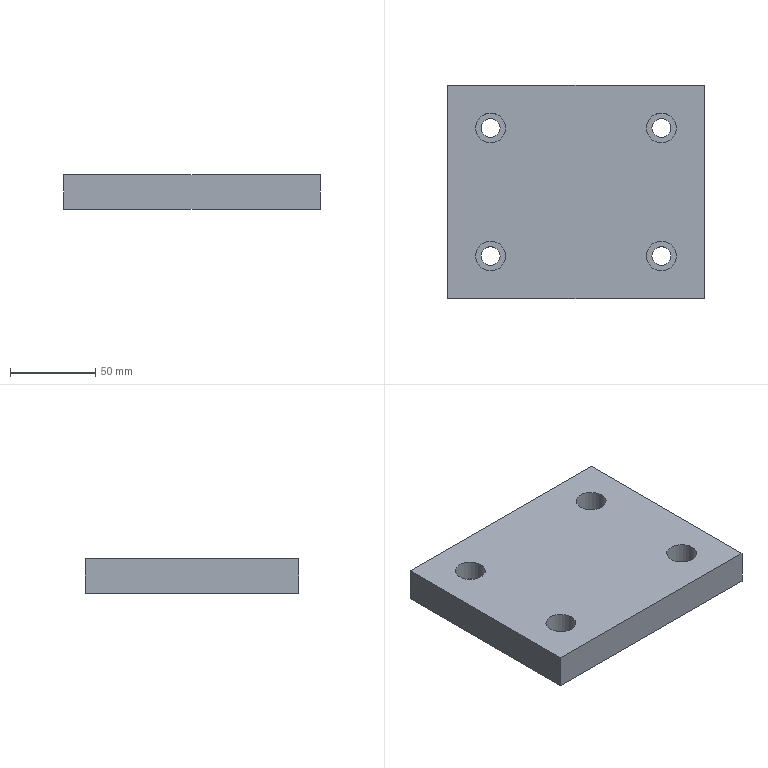Part | NX | features solid 2 | 1 solid | 18 faces | box 150 x 125 x 20 mm | volume 360414 mm3 | plane 10 | cylinder 8 | commonest cylinder face diameters 11 x4 17.5 x4
STEP:
#1=CARTESIAN_POINT('',(504.6,-600.,-350.));
#2=VERTEX_POINT('',#1);
#3=CARTESIAN_POINT('',(504.6,-600.,-370.));
#4=VERTEX_POINT('',#3);
#5=CARTESIAN_POINT('',(504.6,-600.,-350.));
#6=DIRECTION('',(0.,0.,1.));
#7=VECTOR('',#6,1000.);
#8=LINE('',#5,#7);
#9=EDGE_CURVE('',#2,#4,#8,.F.);
#10=ORIENTED_EDGE('',*,*,#9,.T.);
#11=CARTESIAN_POINT('',(354.6,-600.,-370.));
#12=VERTEX_POINT('',#11);
#13=CARTESIAN_POINT('',(504.6,-600.,-370.));
#14=DIRECTION('',(-1.,0.,0.));
#15=VECTOR('',#14,1000.);
#16=LINE('',#13,#15);
#17=EDGE_CURVE('',#4,#12,#16,.T.);
#18=ORIENTED_EDGE('',*,*,#17,.T.);
#19=CARTESIAN_POINT('',(354.6,-600.,-350.));
#20=VERTEX_POINT('',#19);
#21=CARTESIAN_POINT('',(354.6,-600.,-350.));
#22=DIRECTION('',(0.,0.,-1.));
#23=VECTOR('',#22,1000.);
#24=LINE('',#21,#23);
#25=EDGE_CURVE('',#20,#12,#24,.T.);
#26=ORIENTED_EDGE('',*,*,#25,.F.);
#27=CARTESIAN_POINT('',(504.6,-600.,-350.));
#28=DIRECTION('',(-1.,0.,0.));
#29=VECTOR('',#28,1000.);
#30=LINE('',#27,#29);
#31=EDGE_CURVE('',#2,#20,#30,.T.);
#32=ORIENTED_EDGE('',*,*,#31,.F.);
#33=EDGE_LOOP('',(#10,#18,#26,#32));
#34=FACE_BOUND('',#33,.T.);
#35=CARTESIAN_POINT('',(504.6,-600.,-350.));
#36=DIRECTION('',(0.,1.,0.));
#37=DIRECTION('',(-1.,0.,0.));
#38=AXIS2_PLACEMENT_3D('',#35,#36,#37);
#39=PLANE('',#38);
#40=ADVANCED_FACE('',(#34),#39,.T.);
#41=ORIENTED_EDGE('',*,*,#25,.T.);
#42=CARTESIAN_POINT('',(354.6,-725.,-370.));
#43=VERTEX_POINT('',#42);
#44=CARTESIAN_POINT('',(354.6,-600.,-370.));
#45=DIRECTION('',(0.,1.,0.));
#46=VECTOR('',#45,1000.);
#47=LINE('',#44,#46);
#48=EDGE_CURVE('',#12,#43,#47,.F.);
#49=ORIENTED_EDGE('',*,*,#48,.T.);
#50=CARTESIAN_POINT('',(354.6,-725.,-350.));
#51=VERTEX_POINT('',#50);
#52=CARTESIAN_POINT('',(354.6,-725.,-350.));
#53=DIRECTION('',(0.,0.,1.));
#54=VECTOR('',#53,1000.);
#55=LINE('',#52,#54);
#56=EDGE_CURVE('',#51,#43,#55,.F.);
#57=ORIENTED_EDGE('',*,*,#56,.F.);
#58=CARTESIAN_POINT('',(354.6,-600.,-350.));
#59=DIRECTION('',(0.,1.,0.));
#60=VECTOR('',#59,1000.);
#61=LINE('',#58,#60);
#62=EDGE_CURVE('',#20,#51,#61,.F.);
#63=ORIENTED_EDGE('',*,*,#62,.F.);
#64=EDGE_LOOP('',(#41,#49,#57,#63));
#65=FACE_BOUND('',#64,.T.);
#66=CARTESIAN_POINT('',(354.6,-600.,-350.));
#67=DIRECTION('',(-1.,0.,0.));
#68=DIRECTION('',(0.,-1.,0.));
#69=AXIS2_PLACEMENT_3D('',#66,#67,#68);
#70=PLANE('',#69);
#71=ADVANCED_FACE('',(#65),#70,.T.);
#72=ORIENTED_EDGE('',*,*,#56,.T.);
#73=CARTESIAN_POINT('',(504.6,-725.,-370.));
#74=VERTEX_POINT('',#73);
#75=CARTESIAN_POINT('',(504.6,-725.,-370.));
#76=DIRECTION('',(-1.,0.,0.));
#77=VECTOR('',#76,1000.);
#78=LINE('',#75,#77);
#79=EDGE_CURVE('',#74,#43,#78,.T.);
#80=ORIENTED_EDGE('',*,*,#79,.F.);
#81=CARTESIAN_POINT('',(504.6,-725.,-350.));
#82=VERTEX_POINT('',#81);
#83=CARTESIAN_POINT('',(504.6,-725.,-350.));
#84=DIRECTION('',(0.,0.,-1.));
#85=VECTOR('',#84,1000.);
#86=LINE('',#83,#85);
#87=EDGE_CURVE('',#82,#74,#86,.T.);
#88=ORIENTED_EDGE('',*,*,#87,.F.);
#89=CARTESIAN_POINT('',(504.6,-725.,-350.));
#90=DIRECTION('',(-1.,0.,0.));
#91=VECTOR('',#90,1000.);
#92=LINE('',#89,#91);
#93=EDGE_CURVE('',#82,#51,#92,.T.);
#94=ORIENTED_EDGE('',*,*,#93,.T.);
#95=EDGE_LOOP('',(#72,#80,#88,#94));
#96=FACE_BOUND('',#95,.T.);
#97=CARTESIAN_POINT('',(504.6,-725.,-350.));
#98=DIRECTION('',(0.,1.,0.));
#99=DIRECTION('',(-1.,0.,0.));
#100=AXIS2_PLACEMENT_3D('',#97,#98,#99);
#101=PLANE('',#100);
#102=ADVANCED_FACE('',(#96),#101,.F.);
#103=CARTESIAN_POINT('',(504.6,-600.,-350.));
#104=DIRECTION('',(0.,-1.,0.));
#105=VECTOR('',#104,1000.);
#106=LINE('',#103,#105);
#107=EDGE_CURVE('',#2,#82,#106,.T.);
#108=ORIENTED_EDGE('',*,*,#107,.T.);
#109=ORIENTED_EDGE('',*,*,#87,.T.);
#110=CARTESIAN_POINT('',(504.6,-600.,-370.));
#111=DIRECTION('',(0.,-1.,0.));
#112=VECTOR('',#111,1000.);
#113=LINE('',#110,#112);
#114=EDGE_CURVE('',#4,#74,#113,.T.);
#115=ORIENTED_EDGE('',*,*,#114,.F.);
#116=ORIENTED_EDGE('',*,*,#9,.F.);
#117=EDGE_LOOP('',(#108,#109,#115,#116));
#118=FACE_BOUND('',#117,.T.);
#119=CARTESIAN_POINT('',(504.6,-600.,-350.));
#120=DIRECTION('',(-1.,0.,0.));
#121=DIRECTION('',(0.,-1.,0.));
#122=AXIS2_PLACEMENT_3D('',#119,#120,#121);
#123=PLANE('',#122);
#124=ADVANCED_FACE('',(#118),#123,.F.);
#125=CARTESIAN_POINT('',(474.1,-625.,-370.));
#126=VERTEX_POINT('',#125);
#127=CARTESIAN_POINT('',(479.6,-625.,-370.));
#128=DIRECTION('',(0.,0.,1.));
#129=DIRECTION('',(-1.,0.,0.));
#130=AXIS2_PLACEMENT_3D('',#127,#128,#129);
#131=CIRCLE('',#130,5.5);
#132=EDGE_CURVE('',#126,#126,#131,.T.);
#133=ORIENTED_EDGE('',*,*,#132,.T.);
#134=EDGE_LOOP('',(#133));
#135=FACE_BOUND('',#134,.T.);
#136=CARTESIAN_POINT('',(374.1,-625.,-370.));
#137=VERTEX_POINT('',#136);
#138=CARTESIAN_POINT('',(379.6,-625.,-370.));
#139=DIRECTION('',(0.,0.,1.));
#140=DIRECTION('',(-1.,0.,0.));
#141=AXIS2_PLACEMENT_3D('',#138,#139,#140);
#142=CIRCLE('',#141,5.5);
#143=EDGE_CURVE('',#137,#137,#142,.T.);
#144=ORIENTED_EDGE('',*,*,#143,.T.);
#145=EDGE_LOOP('',(#144));
#146=FACE_BOUND('',#145,.T.);
#147=CARTESIAN_POINT('',(474.1,-700.,-370.));
#148=VERTEX_POINT('',#147);
#149=CARTESIAN_POINT('',(479.6,-700.,-370.));
#150=DIRECTION('',(0.,0.,-1.));
#151=DIRECTION('',(-1.,0.,0.));
#152=AXIS2_PLACEMENT_3D('',#149,#150,#151);
#153=CIRCLE('',#152,5.5);
#154=EDGE_CURVE('',#148,#148,#153,.F.);
#155=ORIENTED_EDGE('',*,*,#154,.T.);
#156=EDGE_LOOP('',(#155));
#157=FACE_BOUND('',#156,.T.);
#158=CARTESIAN_POINT('',(374.1,-700.,-370.));
#159=VERTEX_POINT('',#158);
#160=CARTESIAN_POINT('',(379.6,-700.,-370.));
#161=DIRECTION('',(0.,0.,-1.));
#162=DIRECTION('',(-1.,0.,0.));
#163=AXIS2_PLACEMENT_3D('',#160,#161,#162);
#164=CIRCLE('',#163,5.5);
#165=EDGE_CURVE('',#159,#159,#164,.F.);
#166=ORIENTED_EDGE('',*,*,#165,.T.);
#167=EDGE_LOOP('',(#166));
#168=FACE_BOUND('',#167,.T.);
#169=ORIENTED_EDGE('',*,*,#79,.T.);
#170=ORIENTED_EDGE('',*,*,#48,.F.);
#171=ORIENTED_EDGE('',*,*,#17,.F.);
#172=ORIENTED_EDGE('',*,*,#114,.T.);
#173=EDGE_LOOP('',(#169,#170,#171,#172));
#174=FACE_BOUND('',#173,.T.);
#175=CARTESIAN_POINT('',(504.6,-600.,-370.));
#176=DIRECTION('',(0.,0.,1.));
#177=DIRECTION('',(-1.,0.,0.));
#178=AXIS2_PLACEMENT_3D('',#175,#176,#177);
#179=PLANE('',#178);
#180=ADVANCED_FACE('',(#135,#146,#157,#168,#174),#179,.F.);
#181=CARTESIAN_POINT('',(488.35,-625.,-350.));
#182=VERTEX_POINT('',#181);
#183=CARTESIAN_POINT('',(479.6,-625.,-350.));
#184=DIRECTION('',(0.,0.,-1.));
#185=DIRECTION('',(1.,0.,0.));
#186=AXIS2_PLACEMENT_3D('',#183,#184,#185);
#187=CIRCLE('',#186,8.75);
#188=EDGE_CURVE('',#182,#182,#187,.T.);
#189=ORIENTED_EDGE('',*,*,#188,.T.);
#190=EDGE_LOOP('',(#189));
#191=FACE_BOUND('',#190,.T.);
#192=CARTESIAN_POINT('',(388.35,-625.,-350.));
#193=VERTEX_POINT('',#192);
#194=CARTESIAN_POINT('',(379.6,-625.,-350.));
#195=DIRECTION('',(0.,0.,-1.));
#196=DIRECTION('',(1.,0.,0.));
#197=AXIS2_PLACEMENT_3D('',#194,#195,#196);
#198=CIRCLE('',#197,8.75);
#199=EDGE_CURVE('',#193,#193,#198,.T.);
#200=ORIENTED_EDGE('',*,*,#199,.T.);
#201=EDGE_LOOP('',(#200));
#202=FACE_BOUND('',#201,.T.);
#203=CARTESIAN_POINT('',(470.85,-700.,-350.));
#204=VERTEX_POINT('',#203);
#205=CARTESIAN_POINT('',(479.6,-700.,-350.));
#206=DIRECTION('',(0.,0.,-1.));
#207=DIRECTION('',(-1.,0.,0.));
#208=AXIS2_PLACEMENT_3D('',#205,#206,#207);
#209=CIRCLE('',#208,8.75);
#210=EDGE_CURVE('',#204,#204,#209,.T.);
#211=ORIENTED_EDGE('',*,*,#210,.T.);
#212=EDGE_LOOP('',(#211));
#213=FACE_BOUND('',#212,.T.);
#214=CARTESIAN_POINT('',(370.85,-700.,-350.));
#215=VERTEX_POINT('',#214);
#216=CARTESIAN_POINT('',(379.6,-700.,-350.));
#217=DIRECTION('',(0.,0.,-1.));
#218=DIRECTION('',(-1.,0.,0.));
#219=AXIS2_PLACEMENT_3D('',#216,#217,#218);
#220=CIRCLE('',#219,8.75);
#221=EDGE_CURVE('',#215,#215,#220,.T.);
#222=ORIENTED_EDGE('',*,*,#221,.T.);
#223=EDGE_LOOP('',(#222));
#224=FACE_BOUND('',#223,.T.);
#225=ORIENTED_EDGE('',*,*,#93,.F.);
#226=ORIENTED_EDGE('',*,*,#107,.F.);
#227=ORIENTED_EDGE('',*,*,#31,.T.);
#228=ORIENTED_EDGE('',*,*,#62,.T.);
#229=EDGE_LOOP('',(#225,#226,#227,#228));
#230=FACE_BOUND('',#229,.T.);
#231=CARTESIAN_POINT('',(504.6,-600.,-350.));
#232=DIRECTION('',(0.,0.,1.));
#233=DIRECTION('',(-1.,0.,0.));
#234=AXIS2_PLACEMENT_3D('',#231,#232,#233);
#235=PLANE('',#234);
#236=ADVANCED_FACE('',(#191,#202,#213,#224,#230),#235,.T.);
#237=CARTESIAN_POINT('',(385.1,-700.,-362.));
#238=VERTEX_POINT('',#237);
#239=CARTESIAN_POINT('',(379.6,-700.,-362.));
#240=DIRECTION('',(0.,0.,-1.));
#241=DIRECTION('',(1.,0.,0.));
#242=AXIS2_PLACEMENT_3D('',#239,#240,#241);
#243=CIRCLE('',#242,5.5);
#244=EDGE_CURVE('',#238,#238,#243,.T.);
#245=ORIENTED_EDGE('',*,*,#244,.F.);
#246=EDGE_LOOP('',(#245));
#247=FACE_BOUND('',#246,.T.);
#248=ORIENTED_EDGE('',*,*,#165,.F.);
#249=EDGE_LOOP('',(#248));
#250=FACE_BOUND('',#249,.T.);
#251=CARTESIAN_POINT('',(379.6,-700.,-400.));
#252=DIRECTION('',(0.,0.,-1.));
#253=DIRECTION('',(1.,0.,0.));
#254=AXIS2_PLACEMENT_3D('',#251,#252,#253);
#255=CYLINDRICAL_SURFACE('',#254,5.5);
#256=ADVANCED_FACE('',(#247,#250),#255,.F.);
#257=ORIENTED_EDGE('',*,*,#244,.T.);
#258=EDGE_LOOP('',(#257));
#259=FACE_BOUND('',#258,.T.);
#260=CARTESIAN_POINT('',(388.35,-700.,-362.));
#261=VERTEX_POINT('',#260);
#262=CARTESIAN_POINT('',(379.6,-700.,-362.));
#263=DIRECTION('',(0.,0.,-1.));
#264=DIRECTION('',(1.,0.,0.));
#265=AXIS2_PLACEMENT_3D('',#262,#263,#264);
#266=CIRCLE('',#265,8.75);
#267=EDGE_CURVE('',#261,#261,#266,.T.);
#268=ORIENTED_EDGE('',*,*,#267,.F.);
#269=EDGE_LOOP('',(#268));
#270=FACE_BOUND('',#269,.T.);
#271=CARTESIAN_POINT('',(417.1,-700.,-362.));
#272=DIRECTION('',(0.,0.,-1.));
#273=DIRECTION('',(1.,0.,0.));
#274=AXIS2_PLACEMENT_3D('',#271,#272,#273);
#275=PLANE('',#274);
#276=ADVANCED_FACE('',(#259,#270),#275,.F.);
#277=ORIENTED_EDGE('',*,*,#267,.T.);
#278=EDGE_LOOP('',(#277));
#279=FACE_BOUND('',#278,.T.);
#280=ORIENTED_EDGE('',*,*,#221,.F.);
#281=EDGE_LOOP('',(#280));
#282=FACE_BOUND('',#281,.T.);
#283=CARTESIAN_POINT('',(379.6,-700.,-350.));
#284=DIRECTION('',(0.,0.,-1.));
#285=DIRECTION('',(1.,0.,0.));
#286=AXIS2_PLACEMENT_3D('',#283,#284,#285);
#287=CYLINDRICAL_SURFACE('',#286,8.75);
#288=ADVANCED_FACE('',(#279,#282),#287,.F.);
#289=CARTESIAN_POINT('',(485.1,-700.,-362.));
#290=VERTEX_POINT('',#289);
#291=CARTESIAN_POINT('',(479.6,-700.,-362.));
#292=DIRECTION('',(0.,0.,-1.));
#293=DIRECTION('',(1.,0.,0.));
#294=AXIS2_PLACEMENT_3D('',#291,#292,#293);
#295=CIRCLE('',#294,5.5);
#296=EDGE_CURVE('',#290,#290,#295,.T.);
#297=ORIENTED_EDGE('',*,*,#296,.F.);
#298=EDGE_LOOP('',(#297));
#299=FACE_BOUND('',#298,.T.);
#300=ORIENTED_EDGE('',*,*,#154,.F.);
#301=EDGE_LOOP('',(#300));
#302=FACE_BOUND('',#301,.T.);
#303=CARTESIAN_POINT('',(479.6,-700.,-400.));
#304=DIRECTION('',(0.,0.,-1.));
#305=DIRECTION('',(1.,0.,0.));
#306=AXIS2_PLACEMENT_3D('',#303,#304,#305);
#307=CYLINDRICAL_SURFACE('',#306,5.5);
#308=ADVANCED_FACE('',(#299,#302),#307,.F.);
#309=ORIENTED_EDGE('',*,*,#296,.T.);
#310=EDGE_LOOP('',(#309));
#311=FACE_BOUND('',#310,.T.);
#312=CARTESIAN_POINT('',(488.35,-700.,-362.));
#313=VERTEX_POINT('',#312);
#314=CARTESIAN_POINT('',(479.6,-700.,-362.));
#315=DIRECTION('',(0.,0.,-1.));
#316=DIRECTION('',(1.,0.,0.));
#317=AXIS2_PLACEMENT_3D('',#314,#315,#316);
#318=CIRCLE('',#317,8.75);
#319=EDGE_CURVE('',#313,#313,#318,.T.);
#320=ORIENTED_EDGE('',*,*,#319,.F.);
#321=EDGE_LOOP('',(#320));
#322=FACE_BOUND('',#321,.T.);
#323=CARTESIAN_POINT('',(467.1,-700.,-362.));
#324=DIRECTION('',(0.,0.,-1.));
#325=DIRECTION('',(1.,0.,0.));
#326=AXIS2_PLACEMENT_3D('',#323,#324,#325);
#327=PLANE('',#326);
#328=ADVANCED_FACE('',(#311,#322),#327,.F.);
#329=ORIENTED_EDGE('',*,*,#319,.T.);
#330=EDGE_LOOP('',(#329));
#331=FACE_BOUND('',#330,.T.);
#332=ORIENTED_EDGE('',*,*,#210,.F.);
#333=EDGE_LOOP('',(#332));
#334=FACE_BOUND('',#333,.T.);
#335=CARTESIAN_POINT('',(479.6,-700.,-350.));
#336=DIRECTION('',(0.,0.,-1.));
#337=DIRECTION('',(1.,0.,0.));
#338=AXIS2_PLACEMENT_3D('',#335,#336,#337);
#339=CYLINDRICAL_SURFACE('',#338,8.75);
#340=ADVANCED_FACE('',(#331,#334),#339,.F.);
#341=CARTESIAN_POINT('',(385.1,-625.,-362.));
#342=VERTEX_POINT('',#341);
#343=CARTESIAN_POINT('',(379.6,-625.,-362.));
#344=DIRECTION('',(0.,0.,-1.));
#345=DIRECTION('',(1.,0.,0.));
#346=AXIS2_PLACEMENT_3D('',#343,#344,#345);
#347=CIRCLE('',#346,5.5);
#348=EDGE_CURVE('',#342,#342,#347,.T.);
#349=ORIENTED_EDGE('',*,*,#348,.F.);
#350=EDGE_LOOP('',(#349));
#351=FACE_BOUND('',#350,.T.);
#352=ORIENTED_EDGE('',*,*,#143,.F.);
#353=EDGE_LOOP('',(#352));
#354=FACE_BOUND('',#353,.T.);
#355=CARTESIAN_POINT('',(379.6,-625.,-400.));
#356=DIRECTION('',(0.,0.,-1.));
#357=DIRECTION('',(1.,0.,0.));
#358=AXIS2_PLACEMENT_3D('',#355,#356,#357);
#359=CYLINDRICAL_SURFACE('',#358,5.5);
#360=ADVANCED_FACE('',(#351,#354),#359,.F.);
#361=ORIENTED_EDGE('',*,*,#348,.T.);
#362=EDGE_LOOP('',(#361));
#363=FACE_BOUND('',#362,.T.);
#364=CARTESIAN_POINT('',(388.35,-625.,-362.));
#365=VERTEX_POINT('',#364);
#366=CARTESIAN_POINT('',(379.6,-625.,-362.));
#367=DIRECTION('',(0.,0.,-1.));
#368=DIRECTION('',(1.,0.,0.));
#369=AXIS2_PLACEMENT_3D('',#366,#367,#368);
#370=CIRCLE('',#369,8.75);
#371=EDGE_CURVE('',#365,#365,#370,.T.);
#372=ORIENTED_EDGE('',*,*,#371,.F.);
#373=EDGE_LOOP('',(#372));
#374=FACE_BOUND('',#373,.T.);
#375=CARTESIAN_POINT('',(417.1,-625.,-362.));
#376=DIRECTION('',(0.,0.,-1.));
#377=DIRECTION('',(1.,0.,0.));
#378=AXIS2_PLACEMENT_3D('',#375,#376,#377);
#379=PLANE('',#378);
#380=ADVANCED_FACE('',(#363,#374),#379,.F.);
#381=ORIENTED_EDGE('',*,*,#371,.T.);
#382=EDGE_LOOP('',(#381));
#383=FACE_BOUND('',#382,.T.);
#384=ORIENTED_EDGE('',*,*,#199,.F.);
#385=EDGE_LOOP('',(#384));
#386=FACE_BOUND('',#385,.T.);
#387=CARTESIAN_POINT('',(379.6,-625.,-350.));
#388=DIRECTION('',(0.,0.,-1.));
#389=DIRECTION('',(1.,0.,0.));
#390=AXIS2_PLACEMENT_3D('',#387,#388,#389);
#391=CYLINDRICAL_SURFACE('',#390,8.75);
#392=ADVANCED_FACE('',(#383,#386),#391,.F.);
#393=CARTESIAN_POINT('',(485.1,-625.,-362.));
#394=VERTEX_POINT('',#393);
#395=CARTESIAN_POINT('',(479.6,-625.,-362.));
#396=DIRECTION('',(0.,0.,-1.));
#397=DIRECTION('',(1.,0.,0.));
#398=AXIS2_PLACEMENT_3D('',#395,#396,#397);
#399=CIRCLE('',#398,5.5);
#400=EDGE_CURVE('',#394,#394,#399,.T.);
#401=ORIENTED_EDGE('',*,*,#400,.F.);
#402=EDGE_LOOP('',(#401));
#403=FACE_BOUND('',#402,.T.);
#404=ORIENTED_EDGE('',*,*,#132,.F.);
#405=EDGE_LOOP('',(#404));
#406=FACE_BOUND('',#405,.T.);
#407=CARTESIAN_POINT('',(479.6,-625.,-400.));
#408=DIRECTION('',(0.,0.,-1.));
#409=DIRECTION('',(1.,0.,0.));
#410=AXIS2_PLACEMENT_3D('',#407,#408,#409);
#411=CYLINDRICAL_SURFACE('',#410,5.5);
#412=ADVANCED_FACE('',(#403,#406),#411,.F.);
#413=ORIENTED_EDGE('',*,*,#400,.T.);
#414=EDGE_LOOP('',(#413));
#415=FACE_BOUND('',#414,.T.);
#416=CARTESIAN_POINT('',(488.35,-625.,-362.));
#417=VERTEX_POINT('',#416);
#418=CARTESIAN_POINT('',(479.6,-625.,-362.));
#419=DIRECTION('',(0.,0.,-1.));
#420=DIRECTION('',(1.,0.,0.));
#421=AXIS2_PLACEMENT_3D('',#418,#419,#420);
#422=CIRCLE('',#421,8.75);
#423=EDGE_CURVE('',#417,#417,#422,.T.);
#424=ORIENTED_EDGE('',*,*,#423,.F.);
#425=EDGE_LOOP('',(#424));
#426=FACE_BOUND('',#425,.T.);
#427=CARTESIAN_POINT('',(467.1,-625.,-362.));
#428=DIRECTION('',(0.,0.,-1.));
#429=DIRECTION('',(1.,0.,0.));
#430=AXIS2_PLACEMENT_3D('',#427,#428,#429);
#431=PLANE('',#430);
#432=ADVANCED_FACE('',(#415,#426),#431,.F.);
#433=ORIENTED_EDGE('',*,*,#423,.T.);
#434=EDGE_LOOP('',(#433));
#435=FACE_BOUND('',#434,.T.);
#436=ORIENTED_EDGE('',*,*,#188,.F.);
#437=EDGE_LOOP('',(#436));
#438=FACE_BOUND('',#437,.T.);
#439=CARTESIAN_POINT('',(479.6,-625.,-350.));
#440=DIRECTION('',(0.,0.,-1.));
#441=DIRECTION('',(1.,0.,0.));
#442=AXIS2_PLACEMENT_3D('',#439,#440,#441);
#443=CYLINDRICAL_SURFACE('',#442,8.75);
#444=ADVANCED_FACE('',(#435,#438),#443,.F.);
#445=CLOSED_SHELL('',(#40,#71,#102,#124,#180,#236,#256,#276,#288,#308,#328,#340,#360,#380,#392,#412,#432,#444));
#446=MANIFOLD_SOLID_BREP('',#445);
#447=(LENGTH_UNIT()NAMED_UNIT(*)SI_UNIT(.MILLI.,.METRE.));
#448=UNCERTAINTY_MEASURE_WITH_UNIT(LENGTH_MEASURE(0.00001),#447,'','');
#449=(NAMED_UNIT(*)PLANE_ANGLE_UNIT()SI_UNIT($,.RADIAN.));
#450=(NAMED_UNIT(*)SI_UNIT($,.STERADIAN.)SOLID_ANGLE_UNIT());
#451=(GEOMETRIC_REPRESENTATION_CONTEXT(3)GLOBAL_UNCERTAINTY_ASSIGNED_CONTEXT((#448))GLOBAL_UNIT_ASSIGNED_CONTEXT((#447,#449,#450))REPRESENTATION_CONTEXT('',''));
#452=ADVANCED_BREP_SHAPE_REPRESENTATION('',(#446),#451);